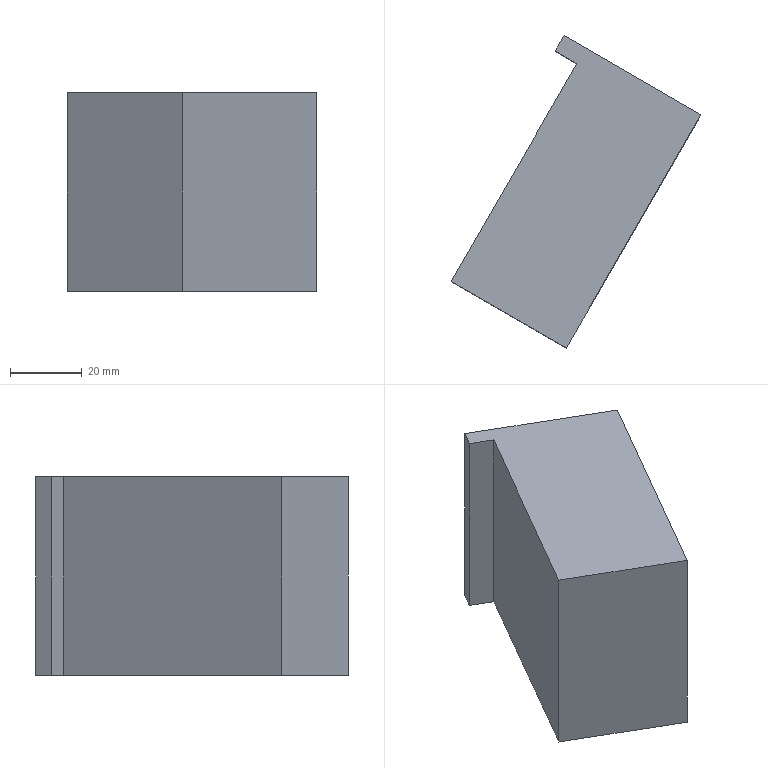Part | NX | features solid 2 | 1 solid | 8 faces | box 69.543 x 86.952 x 55.145 mm | volume 154956 mm3 | plane 8
STEP:
#1=CARTESIAN_POINT('',(430.404,719.447,50.));
#2=VERTEX_POINT('',#1);
#3=CARTESIAN_POINT('',(430.404,719.447,-5.145));
#4=VERTEX_POINT('',#3);
#5=CARTESIAN_POINT('',(430.404,719.447,50.));
#6=DIRECTION('',(0.,0.,-1.));
#7=VECTOR('',#6,1000.);
#8=LINE('',#5,#7);
#9=EDGE_CURVE('',#2,#4,#8,.T.);
#10=ORIENTED_EDGE('',*,*,#9,.T.);
#11=CARTESIAN_POINT('',(427.904,715.117,-5.145));
#12=VERTEX_POINT('',#11);
#13=CARTESIAN_POINT('',(367.904,611.193,-5.145));
#14=DIRECTION('',(0.5,0.866,0.));
#15=VECTOR('',#14,1000.);
#16=LINE('',#13,#15);
#17=EDGE_CURVE('',#12,#4,#16,.T.);
#18=ORIENTED_EDGE('',*,*,#17,.F.);
#19=CARTESIAN_POINT('',(427.904,715.117,50.));
#20=VERTEX_POINT('',#19);
#21=CARTESIAN_POINT('',(427.904,715.117,50.));
#22=DIRECTION('',(0.,0.,-1.));
#23=VECTOR('',#22,1000.);
#24=LINE('',#21,#23);
#25=EDGE_CURVE('',#20,#12,#24,.T.);
#26=ORIENTED_EDGE('',*,*,#25,.F.);
#27=CARTESIAN_POINT('',(400.404,667.485,50.));
#28=DIRECTION('',(-0.5,-0.866,0.));
#29=VECTOR('',#28,1000.);
#30=LINE('',#27,#29);
#31=EDGE_CURVE('',#2,#20,#30,.T.);
#32=ORIENTED_EDGE('',*,*,#31,.F.);
#33=EDGE_LOOP('',(#10,#18,#26,#32));
#34=FACE_BOUND('',#33,.T.);
#35=CARTESIAN_POINT('',(400.404,667.485,50.));
#36=DIRECTION('',(0.866,-0.5,0.));
#37=DIRECTION('',(0.,0.,1.));
#38=AXIS2_PLACEMENT_3D('',#35,#36,#37);
#39=PLANE('',#38);
#40=ADVANCED_FACE('',(#34),#39,.F.);
#41=ORIENTED_EDGE('',*,*,#25,.T.);
#42=CARTESIAN_POINT('',(433.966,711.617,-5.145));
#43=VERTEX_POINT('',#42);
#44=CARTESIAN_POINT('',(465.143,693.617,-5.145));
#45=DIRECTION('',(0.866,-0.5,0.));
#46=VECTOR('',#45,1000.);
#47=LINE('',#44,#46);
#48=EDGE_CURVE('',#12,#43,#47,.T.);
#49=ORIENTED_EDGE('',*,*,#48,.T.);
#50=CARTESIAN_POINT('',(433.966,711.617,50.));
#51=VERTEX_POINT('',#50);
#52=CARTESIAN_POINT('',(433.966,711.617,50.));
#53=DIRECTION('',(0.,0.,-1.));
#54=VECTOR('',#53,1000.);
#55=LINE('',#52,#54);
#56=EDGE_CURVE('',#51,#43,#55,.T.);
#57=ORIENTED_EDGE('',*,*,#56,.F.);
#58=CARTESIAN_POINT('',(465.143,693.617,50.));
#59=DIRECTION('',(0.866,-0.5,0.));
#60=VECTOR('',#59,1000.);
#61=LINE('',#58,#60);
#62=EDGE_CURVE('',#20,#51,#61,.T.);
#63=ORIENTED_EDGE('',*,*,#62,.F.);
#64=EDGE_LOOP('',(#41,#49,#57,#63));
#65=FACE_BOUND('',#64,.T.);
#66=CARTESIAN_POINT('',(465.143,693.617,50.));
#67=DIRECTION('',(0.5,0.866,0.));
#68=DIRECTION('',(0.,0.,1.));
#69=AXIS2_PLACEMENT_3D('',#66,#67,#68);
#70=PLANE('',#69);
#71=ADVANCED_FACE('',(#65),#70,.F.);
#72=ORIENTED_EDGE('',*,*,#56,.T.);
#73=CARTESIAN_POINT('',(398.966,650.995,-5.145));
#74=VERTEX_POINT('',#73);
#75=CARTESIAN_POINT('',(403.966,659.655,-5.145));
#76=DIRECTION('',(-0.5,-0.866,0.));
#77=VECTOR('',#76,1000.);
#78=LINE('',#75,#77);
#79=EDGE_CURVE('',#43,#74,#78,.T.);
#80=ORIENTED_EDGE('',*,*,#79,.T.);
#81=CARTESIAN_POINT('',(398.966,650.995,50.));
#82=VERTEX_POINT('',#81);
#83=CARTESIAN_POINT('',(398.966,650.995,50.));
#84=DIRECTION('',(0.,0.,-1.));
#85=VECTOR('',#84,1000.);
#86=LINE('',#83,#85);
#87=EDGE_CURVE('',#82,#74,#86,.T.);
#88=ORIENTED_EDGE('',*,*,#87,.F.);
#89=CARTESIAN_POINT('',(406.466,663.985,50.));
#90=DIRECTION('',(-0.5,-0.866,0.));
#91=VECTOR('',#90,1000.);
#92=LINE('',#89,#91);
#93=EDGE_CURVE('',#51,#82,#92,.T.);
#94=ORIENTED_EDGE('',*,*,#93,.F.);
#95=EDGE_LOOP('',(#72,#80,#88,#94));
#96=FACE_BOUND('',#95,.T.);
#97=CARTESIAN_POINT('',(406.466,663.985,50.));
#98=DIRECTION('',(0.866,-0.5,0.));
#99=DIRECTION('',(0.,0.,1.));
#100=AXIS2_PLACEMENT_3D('',#97,#98,#99);
#101=PLANE('',#100);
#102=ADVANCED_FACE('',(#96),#101,.F.);
#103=ORIENTED_EDGE('',*,*,#87,.T.);
#104=CARTESIAN_POINT('',(431.009,632.495,-5.145));
#105=VERTEX_POINT('',#104);
#106=CARTESIAN_POINT('',(430.143,632.995,-5.145));
#107=DIRECTION('',(-0.866,0.5,0.));
#108=VECTOR('',#107,1000.);
#109=LINE('',#106,#108);
#110=EDGE_CURVE('',#105,#74,#109,.T.);
#111=ORIENTED_EDGE('',*,*,#110,.F.);
#112=CARTESIAN_POINT('',(431.009,632.495,50.));
#113=VERTEX_POINT('',#112);
#114=CARTESIAN_POINT('',(431.009,632.495,50.));
#115=DIRECTION('',(0.,0.,-1.));
#116=VECTOR('',#115,1000.);
#117=LINE('',#114,#116);
#118=EDGE_CURVE('',#113,#105,#117,.T.);
#119=ORIENTED_EDGE('',*,*,#118,.F.);
#120=CARTESIAN_POINT('',(430.143,632.995,50.));
#121=DIRECTION('',(-0.866,0.5,0.));
#122=VECTOR('',#121,1000.);
#123=LINE('',#120,#122);
#124=EDGE_CURVE('',#113,#82,#123,.T.);
#125=ORIENTED_EDGE('',*,*,#124,.T.);
#126=EDGE_LOOP('',(#103,#111,#119,#125));
#127=FACE_BOUND('',#126,.T.);
#128=CARTESIAN_POINT('',(430.143,632.995,50.));
#129=DIRECTION('',(-0.5,-0.866,0.));
#130=DIRECTION('',(0.,0.,-1.));
#131=AXIS2_PLACEMENT_3D('',#128,#129,#130);
#132=PLANE('',#131);
#133=ADVANCED_FACE('',(#127),#132,.T.);
#134=CARTESIAN_POINT('',(468.509,697.447,50.));
#135=VERTEX_POINT('',#134);
#136=CARTESIAN_POINT('',(467.643,697.947,50.));
#137=DIRECTION('',(-0.866,0.5,0.));
#138=VECTOR('',#137,1000.);
#139=LINE('',#136,#138);
#140=EDGE_CURVE('',#135,#2,#139,.T.);
#141=ORIENTED_EDGE('',*,*,#140,.F.);
#142=CARTESIAN_POINT('',(468.509,697.447,-5.145));
#143=VERTEX_POINT('',#142);
#144=CARTESIAN_POINT('',(468.509,697.447,50.));
#145=DIRECTION('',(0.,0.,-1.));
#146=VECTOR('',#145,1000.);
#147=LINE('',#144,#146);
#148=EDGE_CURVE('',#135,#143,#147,.T.);
#149=ORIENTED_EDGE('',*,*,#148,.T.);
#150=CARTESIAN_POINT('',(467.643,697.947,-5.145));
#151=DIRECTION('',(-0.866,0.5,0.));
#152=VECTOR('',#151,1000.);
#153=LINE('',#150,#152);
#154=EDGE_CURVE('',#143,#4,#153,.T.);
#155=ORIENTED_EDGE('',*,*,#154,.T.);
#156=ORIENTED_EDGE('',*,*,#9,.F.);
#157=EDGE_LOOP('',(#141,#149,#155,#156));
#158=FACE_BOUND('',#157,.T.);
#159=CARTESIAN_POINT('',(467.643,697.947,50.));
#160=DIRECTION('',(-0.5,-0.866,0.));
#161=DIRECTION('',(0.,0.,-1.));
#162=AXIS2_PLACEMENT_3D('',#159,#160,#161);
#163=PLANE('',#162);
#164=ADVANCED_FACE('',(#158),#163,.F.);
#165=ORIENTED_EDGE('',*,*,#31,.T.);
#166=ORIENTED_EDGE('',*,*,#62,.T.);
#167=ORIENTED_EDGE('',*,*,#93,.T.);
#168=ORIENTED_EDGE('',*,*,#124,.F.);
#169=CARTESIAN_POINT('',(438.509,645.485,50.));
#170=DIRECTION('',(-0.5,-0.866,0.));
#171=VECTOR('',#170,1000.);
#172=LINE('',#169,#171);
#173=EDGE_CURVE('',#135,#113,#172,.T.);
#174=ORIENTED_EDGE('',*,*,#173,.F.);
#175=ORIENTED_EDGE('',*,*,#140,.T.);
#176=EDGE_LOOP('',(#165,#166,#167,#168,#174,#175));
#177=FACE_BOUND('',#176,.T.);
#178=CARTESIAN_POINT('',(437.643,645.985,50.));
#179=DIRECTION('',(0.,0.,-1.));
#180=DIRECTION('',(0.5,0.866,0.));
#181=AXIS2_PLACEMENT_3D('',#178,#179,#180);
#182=PLANE('',#181);
#183=ADVANCED_FACE('',(#177),#182,.F.);
#184=ORIENTED_EDGE('',*,*,#79,.F.);
#185=ORIENTED_EDGE('',*,*,#48,.F.);
#186=ORIENTED_EDGE('',*,*,#17,.T.);
#187=ORIENTED_EDGE('',*,*,#154,.F.);
#188=CARTESIAN_POINT('',(406.009,589.193,-5.145));
#189=DIRECTION('',(0.5,0.866,0.));
#190=VECTOR('',#189,1000.);
#191=LINE('',#188,#190);
#192=EDGE_CURVE('',#105,#143,#191,.T.);
#193=ORIENTED_EDGE('',*,*,#192,.F.);
#194=ORIENTED_EDGE('',*,*,#110,.T.);
#195=EDGE_LOOP('',(#184,#185,#186,#187,#193,#194));
#196=FACE_BOUND('',#195,.T.);
#197=CARTESIAN_POINT('',(405.143,589.693,-5.145));
#198=DIRECTION('',(0.,0.,1.));
#199=DIRECTION('',(-0.5,-0.866,0.));
#200=AXIS2_PLACEMENT_3D('',#197,#198,#199);
#201=PLANE('',#200);
#202=ADVANCED_FACE('',(#196),#201,.F.);
#203=ORIENTED_EDGE('',*,*,#118,.T.);
#204=ORIENTED_EDGE('',*,*,#192,.T.);
#205=ORIENTED_EDGE('',*,*,#148,.F.);
#206=ORIENTED_EDGE('',*,*,#173,.T.);
#207=EDGE_LOOP('',(#203,#204,#205,#206));
#208=FACE_BOUND('',#207,.T.);
#209=CARTESIAN_POINT('',(438.509,645.485,50.));
#210=DIRECTION('',(0.866,-0.5,0.));
#211=DIRECTION('',(0.,0.,1.));
#212=AXIS2_PLACEMENT_3D('',#209,#210,#211);
#213=PLANE('',#212);
#214=ADVANCED_FACE('',(#208),#213,.T.);
#215=CLOSED_SHELL('',(#40,#71,#102,#133,#164,#183,#202,#214));
#216=MANIFOLD_SOLID_BREP('',#215);
#217=(LENGTH_UNIT()NAMED_UNIT(*)SI_UNIT(.MILLI.,.METRE.));
#218=UNCERTAINTY_MEASURE_WITH_UNIT(LENGTH_MEASURE(0.00001),#217,'','');
#219=(NAMED_UNIT(*)PLANE_ANGLE_UNIT()SI_UNIT($,.RADIAN.));
#220=(NAMED_UNIT(*)SI_UNIT($,.STERADIAN.)SOLID_ANGLE_UNIT());
#221=(GEOMETRIC_REPRESENTATION_CONTEXT(3)GLOBAL_UNCERTAINTY_ASSIGNED_CONTEXT((#218))GLOBAL_UNIT_ASSIGNED_CONTEXT((#217,#219,#220))REPRESENTATION_CONTEXT('',''));
#222=ADVANCED_BREP_SHAPE_REPRESENTATION('',(#216),#221);